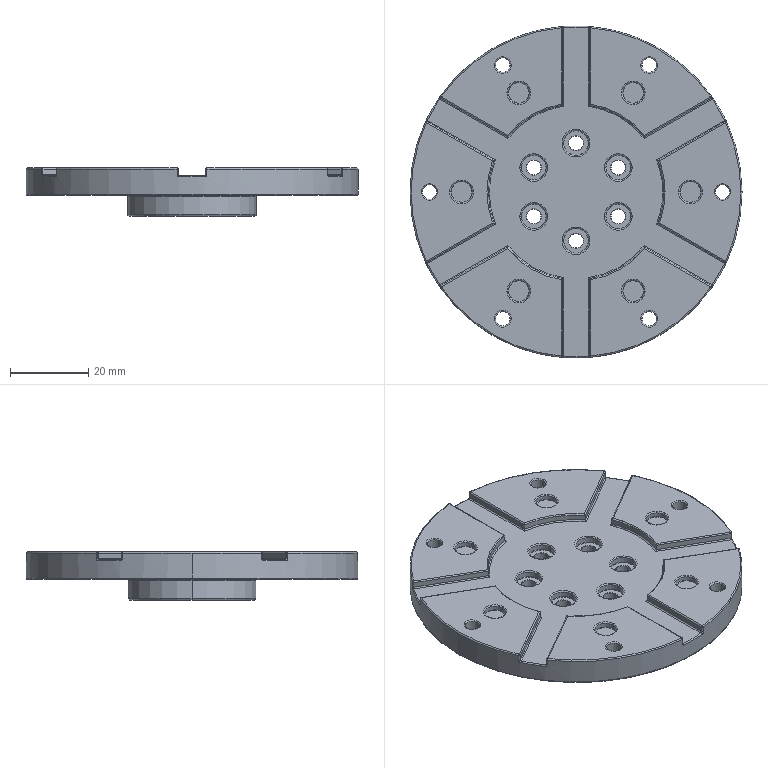Part | SolidWorks | features ICE 7, Fillet 2, Extrusion 1 | 1 solid | 398 faces | box 85 x 85 x 12.3 mm | volume 37399 mm3 | cylinder 169 | torus 129 | plane 75 | sphere 13 | spline 12 | commonest cylinder face diameters 0.6 x74 0.2 x36 3.7 x24 5.5 x12 6.5 x12 45 x7